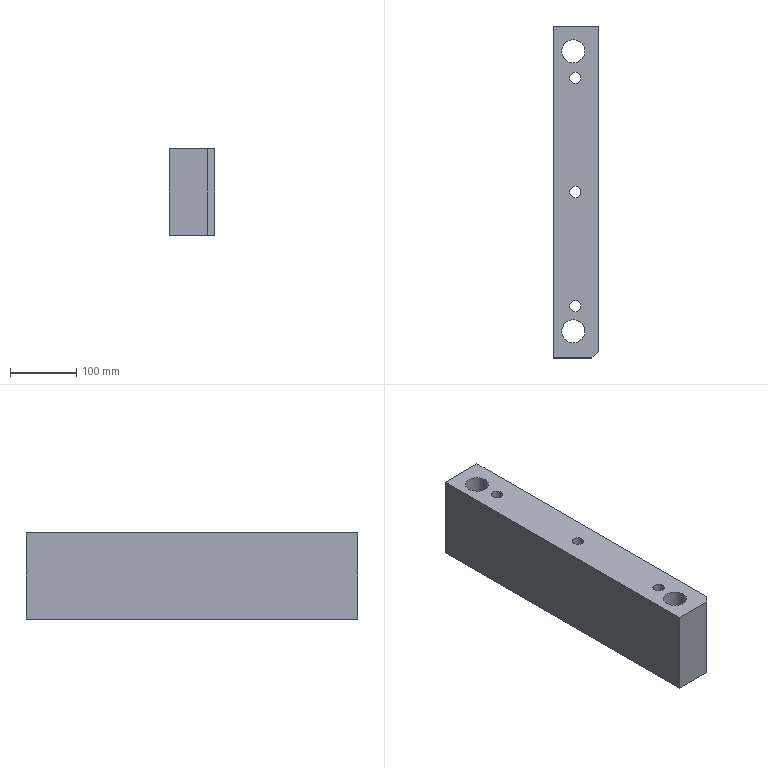Part | STEP file | SL2-MOLD_id742_xmt_txt | 1 solid | 12 faces | box 68 x 500 x 130 mm | volume 4074828 mm3 | plane 7 | cylinder 5 | commonest cylinder face diameters 17 x3 35 x2
STEP:
#1=CARTESIAN_POINT('',(173.5,90.,-244.));
#2=VERTEX_POINT('',#1);
#3=CARTESIAN_POINT('',(165.,90.,-244.));
#4=DIRECTION('',(0.,0.,1.));
#5=DIRECTION('',(1.,0.,0.));
#6=AXIS2_PLACEMENT_3D('',#3,#4,#5);
#7=CIRCLE('',#6,8.5);
#8=EDGE_CURVE('',#2,#2,#7,.T.);
#9=ORIENTED_EDGE('',*,*,#8,.T.);
#10=EDGE_LOOP('',(#9));
#11=FACE_BOUND('',#10,.T.);
#12=CARTESIAN_POINT('',(173.5,-82.,-244.));
#13=VERTEX_POINT('',#12);
#14=CARTESIAN_POINT('',(165.,-82.,-244.));
#15=DIRECTION('',(0.,0.,1.));
#16=DIRECTION('',(1.,0.,0.));
#17=AXIS2_PLACEMENT_3D('',#14,#15,#16);
#18=CIRCLE('',#17,8.5);
#19=EDGE_CURVE('',#13,#13,#18,.T.);
#20=ORIENTED_EDGE('',*,*,#19,.T.);
#21=EDGE_LOOP('',(#20));
#22=FACE_BOUND('',#21,.T.);
#23=CARTESIAN_POINT('',(173.5,262.,-244.));
#24=VERTEX_POINT('',#23);
#25=CARTESIAN_POINT('',(165.,262.,-244.));
#26=DIRECTION('',(0.,0.,1.));
#27=DIRECTION('',(1.,0.,0.));
#28=AXIS2_PLACEMENT_3D('',#25,#26,#27);
#29=CIRCLE('',#28,8.5);
#30=EDGE_CURVE('',#24,#24,#29,.T.);
#31=ORIENTED_EDGE('',*,*,#30,.T.);
#32=EDGE_LOOP('',(#31));
#33=FACE_BOUND('',#32,.T.);
#34=CARTESIAN_POINT('',(179.5,302.,-244.));
#35=VERTEX_POINT('',#34);
#36=CARTESIAN_POINT('',(162.,302.,-244.));
#37=DIRECTION('',(0.,0.,-1.));
#38=DIRECTION('',(1.,0.,0.));
#39=AXIS2_PLACEMENT_3D('',#36,#37,#38);
#40=CIRCLE('',#39,17.5);
#41=EDGE_CURVE('',#35,#35,#40,.T.);
#42=ORIENTED_EDGE('',*,*,#41,.F.);
#43=EDGE_LOOP('',(#42));
#44=FACE_BOUND('',#43,.T.);
#45=CARTESIAN_POINT('',(200.,-150.,-244.));
#46=VERTEX_POINT('',#45);
#47=CARTESIAN_POINT('',(200.,340.,-244.));
#48=VERTEX_POINT('',#47);
#49=CARTESIAN_POINT('',(200.,0.,-244.));
#50=DIRECTION('',(0.,1.,0.));
#51=VECTOR('',#50,1.);
#52=LINE('',#49,#51);
#53=EDGE_CURVE('',#46,#48,#52,.T.);
#54=ORIENTED_EDGE('',*,*,#53,.F.);
#55=CARTESIAN_POINT('',(190.,-160.,-244.));
#56=VERTEX_POINT('',#55);
#57=CARTESIAN_POINT('',(190.,-160.,-244.));
#58=DIRECTION('',(-0.7071,-0.7071,0.));
#59=VECTOR('',#58,1.);
#60=LINE('',#57,#59);
#61=EDGE_CURVE('',#46,#56,#60,.T.);
#62=ORIENTED_EDGE('',*,*,#61,.T.);
#63=CARTESIAN_POINT('',(132.,-160.,-244.));
#64=VERTEX_POINT('',#63);
#65=CARTESIAN_POINT('',(0.,-160.,-244.));
#66=DIRECTION('',(1.,0.,0.));
#67=VECTOR('',#66,1.);
#68=LINE('',#65,#67);
#69=EDGE_CURVE('',#64,#56,#68,.T.);
#70=ORIENTED_EDGE('',*,*,#69,.F.);
#71=CARTESIAN_POINT('',(132.,340.,-244.));
#72=VERTEX_POINT('',#71);
#73=CARTESIAN_POINT('',(132.,0.,-244.));
#74=DIRECTION('',(0.,-1.,0.));
#75=VECTOR('',#74,1.);
#76=LINE('',#73,#75);
#77=EDGE_CURVE('',#72,#64,#76,.T.);
#78=ORIENTED_EDGE('',*,*,#77,.F.);
#79=CARTESIAN_POINT('',(0.,340.,-244.));
#80=DIRECTION('',(-1.,0.,0.));
#81=VECTOR('',#80,1.);
#82=LINE('',#79,#81);
#83=EDGE_CURVE('',#48,#72,#82,.T.);
#84=ORIENTED_EDGE('',*,*,#83,.F.);
#85=EDGE_LOOP('',(#54,#62,#70,#78,#84));
#86=FACE_BOUND('',#85,.T.);
#87=CARTESIAN_POINT('',(179.5,-120.,-244.));
#88=VERTEX_POINT('',#87);
#89=CARTESIAN_POINT('',(162.,-120.,-244.));
#90=DIRECTION('',(0.,0.,-1.));
#91=DIRECTION('',(1.,0.,0.));
#92=AXIS2_PLACEMENT_3D('',#89,#90,#91);
#93=CIRCLE('',#92,17.5);
#94=EDGE_CURVE('',#88,#88,#93,.T.);
#95=ORIENTED_EDGE('',*,*,#94,.F.);
#96=EDGE_LOOP('',(#95));
#97=FACE_BOUND('',#96,.T.);
#98=CARTESIAN_POINT('',(0.,0.,-244.));
#99=DIRECTION('',(0.,0.,1.));
#100=DIRECTION('',(1.,0.,0.));
#101=AXIS2_PLACEMENT_3D('',#98,#99,#100);
#102=PLANE('',#101);
#103=ADVANCED_FACE('',(#11,#22,#33,#44,#86,#97),#102,.F.);
#104=ORIENTED_EDGE('',*,*,#69,.T.);
#105=CARTESIAN_POINT('',(190.,-160.,-114.));
#106=VERTEX_POINT('',#105);
#107=CARTESIAN_POINT('',(190.,-160.,-244.));
#108=DIRECTION('',(0.,0.,1.));
#109=VECTOR('',#108,1.);
#110=LINE('',#107,#109);
#111=EDGE_CURVE('',#56,#106,#110,.T.);
#112=ORIENTED_EDGE('',*,*,#111,.T.);
#113=CARTESIAN_POINT('',(132.,-160.,-114.));
#114=VERTEX_POINT('',#113);
#115=CARTESIAN_POINT('',(0.,-160.,-114.));
#116=DIRECTION('',(1.,0.,0.));
#117=VECTOR('',#116,1.);
#118=LINE('',#115,#117);
#119=EDGE_CURVE('',#114,#106,#118,.T.);
#120=ORIENTED_EDGE('',*,*,#119,.F.);
#121=CARTESIAN_POINT('',(132.,-160.,-244.));
#122=DIRECTION('',(0.,0.,1.));
#123=VECTOR('',#122,1.);
#124=LINE('',#121,#123);
#125=EDGE_CURVE('',#64,#114,#124,.T.);
#126=ORIENTED_EDGE('',*,*,#125,.F.);
#127=EDGE_LOOP('',(#104,#112,#120,#126));
#128=FACE_OUTER_BOUND('',#127,.T.);
#129=CARTESIAN_POINT('',(0.,-160.,-244.));
#130=DIRECTION('',(0.,-1.,0.));
#131=DIRECTION('',(0.,0.,-1.));
#132=AXIS2_PLACEMENT_3D('',#129,#130,#131);
#133=PLANE('',#132);
#134=ADVANCED_FACE('',(#128),#133,.T.);
#135=CARTESIAN_POINT('',(132.,340.,-114.));
#136=VERTEX_POINT('',#135);
#137=CARTESIAN_POINT('',(132.,340.,-244.));
#138=DIRECTION('',(0.,0.,1.));
#139=VECTOR('',#138,1.);
#140=LINE('',#137,#139);
#141=EDGE_CURVE('',#72,#136,#140,.T.);
#142=ORIENTED_EDGE('',*,*,#141,.T.);
#143=CARTESIAN_POINT('',(200.,340.,-114.));
#144=VERTEX_POINT('',#143);
#145=CARTESIAN_POINT('',(0.,340.,-114.));
#146=DIRECTION('',(-1.,0.,0.));
#147=VECTOR('',#146,1.);
#148=LINE('',#145,#147);
#149=EDGE_CURVE('',#144,#136,#148,.T.);
#150=ORIENTED_EDGE('',*,*,#149,.F.);
#151=CARTESIAN_POINT('',(200.,340.,-244.));
#152=DIRECTION('',(0.,0.,1.));
#153=VECTOR('',#152,1.);
#154=LINE('',#151,#153);
#155=EDGE_CURVE('',#48,#144,#154,.T.);
#156=ORIENTED_EDGE('',*,*,#155,.F.);
#157=ORIENTED_EDGE('',*,*,#83,.T.);
#158=EDGE_LOOP('',(#142,#150,#156,#157));
#159=FACE_OUTER_BOUND('',#158,.T.);
#160=CARTESIAN_POINT('',(0.,340.,-244.));
#161=DIRECTION('',(0.,1.,0.));
#162=DIRECTION('',(0.,0.,1.));
#163=AXIS2_PLACEMENT_3D('',#160,#161,#162);
#164=PLANE('',#163);
#165=ADVANCED_FACE('',(#159),#164,.T.);
#166=CARTESIAN_POINT('',(200.,-150.,-114.));
#167=VERTEX_POINT('',#166);
#168=CARTESIAN_POINT('',(200.,0.,-114.));
#169=DIRECTION('',(0.,1.,0.));
#170=VECTOR('',#169,1.);
#171=LINE('',#168,#170);
#172=EDGE_CURVE('',#167,#144,#171,.T.);
#173=ORIENTED_EDGE('',*,*,#172,.F.);
#174=CARTESIAN_POINT('',(200.,-150.,-244.));
#175=DIRECTION('',(0.,0.,-1.));
#176=VECTOR('',#175,1.);
#177=LINE('',#174,#176);
#178=EDGE_CURVE('',#167,#46,#177,.T.);
#179=ORIENTED_EDGE('',*,*,#178,.T.);
#180=ORIENTED_EDGE('',*,*,#53,.T.);
#181=ORIENTED_EDGE('',*,*,#155,.T.);
#182=EDGE_LOOP('',(#173,#179,#180,#181));
#183=FACE_OUTER_BOUND('',#182,.T.);
#184=CARTESIAN_POINT('',(200.,0.,-244.));
#185=DIRECTION('',(1.,0.,0.));
#186=DIRECTION('',(0.,0.,-1.));
#187=AXIS2_PLACEMENT_3D('',#184,#185,#186);
#188=PLANE('',#187);
#189=ADVANCED_FACE('',(#183),#188,.T.);
#190=CARTESIAN_POINT('',(173.5,90.,-114.));
#191=VERTEX_POINT('',#190);
#192=CARTESIAN_POINT('',(165.,90.,-114.));
#193=DIRECTION('',(0.,0.,1.));
#194=DIRECTION('',(1.,0.,0.));
#195=AXIS2_PLACEMENT_3D('',#192,#193,#194);
#196=CIRCLE('',#195,8.5);
#197=EDGE_CURVE('',#191,#191,#196,.T.);
#198=ORIENTED_EDGE('',*,*,#197,.F.);
#199=EDGE_LOOP('',(#198));
#200=FACE_BOUND('',#199,.T.);
#201=CARTESIAN_POINT('',(173.5,-82.,-114.));
#202=VERTEX_POINT('',#201);
#203=CARTESIAN_POINT('',(165.,-82.,-114.));
#204=DIRECTION('',(0.,0.,1.));
#205=DIRECTION('',(1.,0.,0.));
#206=AXIS2_PLACEMENT_3D('',#203,#204,#205);
#207=CIRCLE('',#206,8.5);
#208=EDGE_CURVE('',#202,#202,#207,.T.);
#209=ORIENTED_EDGE('',*,*,#208,.F.);
#210=EDGE_LOOP('',(#209));
#211=FACE_BOUND('',#210,.T.);
#212=CARTESIAN_POINT('',(173.5,262.,-114.));
#213=VERTEX_POINT('',#212);
#214=CARTESIAN_POINT('',(165.,262.,-114.));
#215=DIRECTION('',(0.,0.,1.));
#216=DIRECTION('',(1.,0.,0.));
#217=AXIS2_PLACEMENT_3D('',#214,#215,#216);
#218=CIRCLE('',#217,8.5);
#219=EDGE_CURVE('',#213,#213,#218,.T.);
#220=ORIENTED_EDGE('',*,*,#219,.F.);
#221=EDGE_LOOP('',(#220));
#222=FACE_BOUND('',#221,.T.);
#223=CARTESIAN_POINT('',(179.5,-120.,-114.));
#224=VERTEX_POINT('',#223);
#225=CARTESIAN_POINT('',(162.,-120.,-114.));
#226=DIRECTION('',(0.,0.,-1.));
#227=DIRECTION('',(1.,0.,0.));
#228=AXIS2_PLACEMENT_3D('',#225,#226,#227);
#229=CIRCLE('',#228,17.5);
#230=EDGE_CURVE('',#224,#224,#229,.T.);
#231=ORIENTED_EDGE('',*,*,#230,.T.);
#232=EDGE_LOOP('',(#231));
#233=FACE_BOUND('',#232,.T.);
#234=CARTESIAN_POINT('',(179.5,302.,-114.));
#235=VERTEX_POINT('',#234);
#236=CARTESIAN_POINT('',(162.,302.,-114.));
#237=DIRECTION('',(0.,0.,-1.));
#238=DIRECTION('',(1.,0.,0.));
#239=AXIS2_PLACEMENT_3D('',#236,#237,#238);
#240=CIRCLE('',#239,17.5);
#241=EDGE_CURVE('',#235,#235,#240,.T.);
#242=ORIENTED_EDGE('',*,*,#241,.T.);
#243=EDGE_LOOP('',(#242));
#244=FACE_BOUND('',#243,.T.);
#245=ORIENTED_EDGE('',*,*,#119,.T.);
#246=CARTESIAN_POINT('',(175.,-175.,-114.));
#247=DIRECTION('',(0.7071,0.7071,0.));
#248=VECTOR('',#247,1.);
#249=LINE('',#246,#248);
#250=EDGE_CURVE('',#106,#167,#249,.T.);
#251=ORIENTED_EDGE('',*,*,#250,.T.);
#252=ORIENTED_EDGE('',*,*,#172,.T.);
#253=ORIENTED_EDGE('',*,*,#149,.T.);
#254=CARTESIAN_POINT('',(132.,0.,-114.));
#255=DIRECTION('',(0.,-1.,0.));
#256=VECTOR('',#255,1.);
#257=LINE('',#254,#256);
#258=EDGE_CURVE('',#136,#114,#257,.T.);
#259=ORIENTED_EDGE('',*,*,#258,.T.);
#260=EDGE_LOOP('',(#245,#251,#252,#253,#259));
#261=FACE_BOUND('',#260,.T.);
#262=CARTESIAN_POINT('',(0.,0.,-114.));
#263=DIRECTION('',(0.,0.,1.));
#264=DIRECTION('',(1.,0.,0.));
#265=AXIS2_PLACEMENT_3D('',#262,#263,#264);
#266=PLANE('',#265);
#267=ADVANCED_FACE('',(#200,#211,#222,#233,#244,#261),#266,.T.);
#268=ORIENTED_EDGE('',*,*,#125,.T.);
#269=ORIENTED_EDGE('',*,*,#258,.F.);
#270=ORIENTED_EDGE('',*,*,#141,.F.);
#271=ORIENTED_EDGE('',*,*,#77,.T.);
#272=EDGE_LOOP('',(#268,#269,#270,#271));
#273=FACE_OUTER_BOUND('',#272,.T.);
#274=CARTESIAN_POINT('',(132.,90.,-179.));
#275=DIRECTION('',(1.,0.,0.));
#276=DIRECTION('',(0.,0.,-1.));
#277=AXIS2_PLACEMENT_3D('',#274,#275,#276);
#278=PLANE('',#277);
#279=ADVANCED_FACE('',(#273),#278,.F.);
#280=ORIENTED_EDGE('',*,*,#61,.F.);
#281=ORIENTED_EDGE('',*,*,#178,.F.);
#282=ORIENTED_EDGE('',*,*,#250,.F.);
#283=ORIENTED_EDGE('',*,*,#111,.F.);
#284=EDGE_LOOP('',(#280,#281,#282,#283));
#285=FACE_OUTER_BOUND('',#284,.T.);
#286=CARTESIAN_POINT('',(190.,-160.,-244.));
#287=DIRECTION('',(-0.7071,0.7071,0.));
#288=DIRECTION('',(0.,0.,1.));
#289=AXIS2_PLACEMENT_3D('',#286,#287,#288);
#290=PLANE('',#289);
#291=ADVANCED_FACE('',(#285),#290,.F.);
#292=ORIENTED_EDGE('',*,*,#241,.F.);
#293=EDGE_LOOP('',(#292));
#294=FACE_BOUND('',#293,.T.);
#295=ORIENTED_EDGE('',*,*,#41,.T.);
#296=EDGE_LOOP('',(#295));
#297=FACE_BOUND('',#296,.T.);
#298=CARTESIAN_POINT('',(162.,302.,3221.8));
#299=DIRECTION('',(0.,0.,-1.));
#300=DIRECTION('',(-1.,0.,0.));
#301=AXIS2_PLACEMENT_3D('',#298,#299,#300);
#302=CYLINDRICAL_SURFACE('',#301,17.5);
#303=ADVANCED_FACE('',(#294,#297),#302,.F.);
#304=ORIENTED_EDGE('',*,*,#230,.F.);
#305=EDGE_LOOP('',(#304));
#306=FACE_BOUND('',#305,.T.);
#307=ORIENTED_EDGE('',*,*,#94,.T.);
#308=EDGE_LOOP('',(#307));
#309=FACE_BOUND('',#308,.T.);
#310=CARTESIAN_POINT('',(162.,-120.,3221.8));
#311=DIRECTION('',(0.,0.,-1.));
#312=DIRECTION('',(-1.,0.,0.));
#313=AXIS2_PLACEMENT_3D('',#310,#311,#312);
#314=CYLINDRICAL_SURFACE('',#313,17.5);
#315=ADVANCED_FACE('',(#306,#309),#314,.F.);
#316=ORIENTED_EDGE('',*,*,#219,.T.);
#317=EDGE_LOOP('',(#316));
#318=FACE_BOUND('',#317,.T.);
#319=ORIENTED_EDGE('',*,*,#30,.F.);
#320=EDGE_LOOP('',(#319));
#321=FACE_BOUND('',#320,.T.);
#322=CARTESIAN_POINT('',(165.,262.,-2215.55));
#323=DIRECTION('',(0.,0.,1.));
#324=DIRECTION('',(1.,0.,0.));
#325=AXIS2_PLACEMENT_3D('',#322,#323,#324);
#326=CYLINDRICAL_SURFACE('',#325,8.5);
#327=ADVANCED_FACE('',(#318,#321),#326,.F.);
#328=ORIENTED_EDGE('',*,*,#208,.T.);
#329=EDGE_LOOP('',(#328));
#330=FACE_BOUND('',#329,.T.);
#331=ORIENTED_EDGE('',*,*,#19,.F.);
#332=EDGE_LOOP('',(#331));
#333=FACE_BOUND('',#332,.T.);
#334=CARTESIAN_POINT('',(165.,-82.,-2215.55));
#335=DIRECTION('',(0.,0.,1.));
#336=DIRECTION('',(1.,0.,0.));
#337=AXIS2_PLACEMENT_3D('',#334,#335,#336);
#338=CYLINDRICAL_SURFACE('',#337,8.5);
#339=ADVANCED_FACE('',(#330,#333),#338,.F.);
#340=ORIENTED_EDGE('',*,*,#197,.T.);
#341=EDGE_LOOP('',(#340));
#342=FACE_BOUND('',#341,.T.);
#343=ORIENTED_EDGE('',*,*,#8,.F.);
#344=EDGE_LOOP('',(#343));
#345=FACE_BOUND('',#344,.T.);
#346=CARTESIAN_POINT('',(165.,90.,-2215.55));
#347=DIRECTION('',(0.,0.,1.));
#348=DIRECTION('',(1.,0.,0.));
#349=AXIS2_PLACEMENT_3D('',#346,#347,#348);
#350=CYLINDRICAL_SURFACE('',#349,8.5);
#351=ADVANCED_FACE('',(#342,#345),#350,.F.);
#352=CLOSED_SHELL('',(#103,#134,#165,#189,#267,#279,#291,#303,#315,#327,#339,#351));
#353=MANIFOLD_SOLID_BREP('',#352);
#354=(LENGTH_UNIT()NAMED_UNIT(*)SI_UNIT(.MILLI.,.METRE.));
#355=UNCERTAINTY_MEASURE_WITH_UNIT(LENGTH_MEASURE(0.00002),#354,'','');
#356=(NAMED_UNIT(*)PLANE_ANGLE_UNIT()SI_UNIT($,.RADIAN.));
#357=PLANE_ANGLE_MEASURE_WITH_UNIT(PLANE_ANGLE_MEASURE(0.01745),#356);
#358=DIMENSIONAL_EXPONENTS(0.,0.,0.,0.,0.,0.,0.);
#359=(CONVERSION_BASED_UNIT('DEGREE',#357)NAMED_UNIT(#358)PLANE_ANGLE_UNIT());
#360=(NAMED_UNIT(*)SI_UNIT($,.STERADIAN.)SOLID_ANGLE_UNIT());
#361=(GEOMETRIC_REPRESENTATION_CONTEXT(3)GLOBAL_UNCERTAINTY_ASSIGNED_CONTEXT((#355))GLOBAL_UNIT_ASSIGNED_CONTEXT((#354,#359,#360))REPRESENTATION_CONTEXT('',''));
#362=ADVANCED_BREP_SHAPE_REPRESENTATION('',(#353),#361);